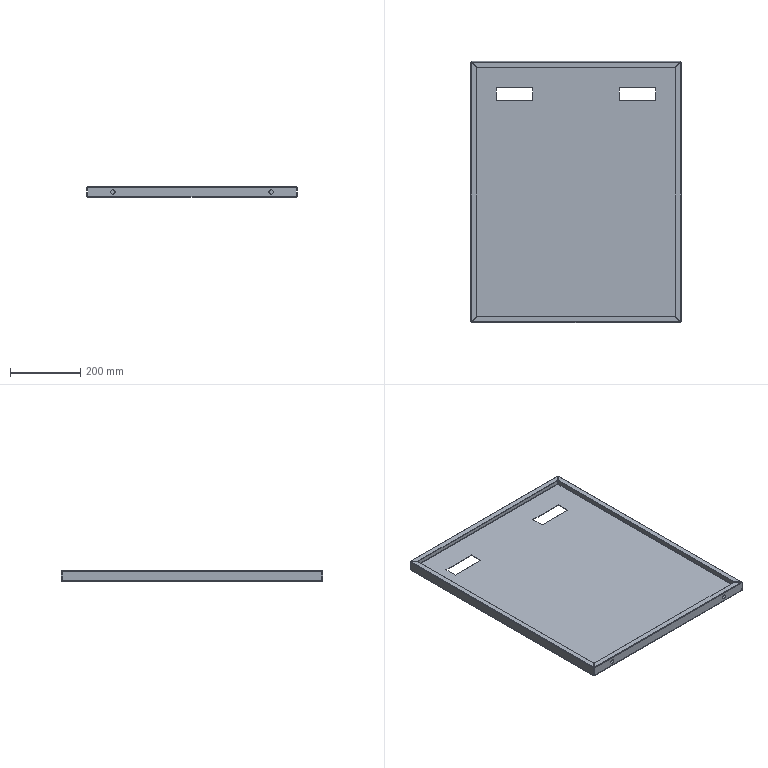Part | NX | 1 solid | 80 faces | box 598 x 743 x 30 mm | volume 822060 mm3 | plane 46 | cylinder 18 | spline 16 | commonest cylinder face diameters 1.473 x8 4.473 x8 12 x2